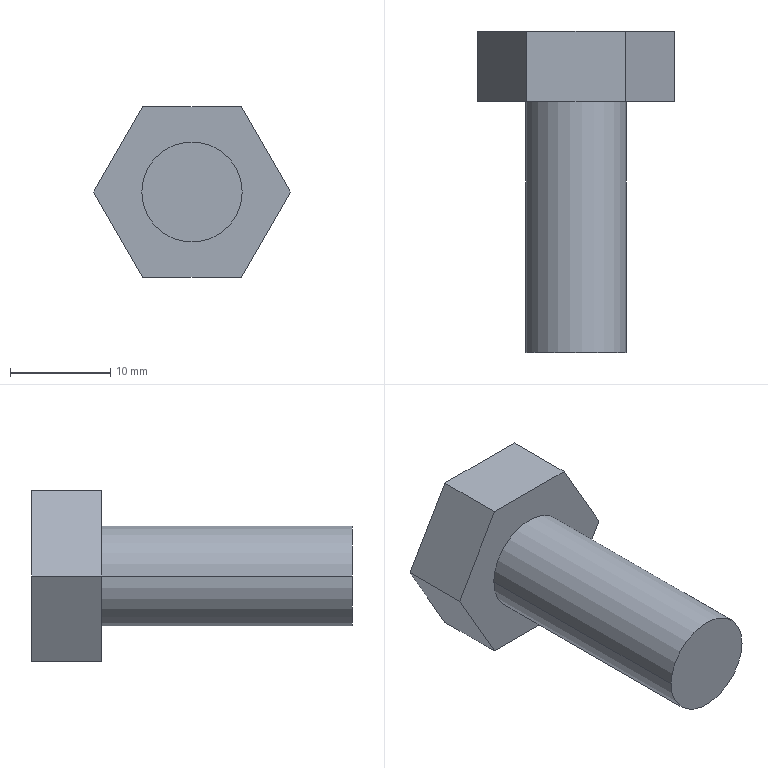Part | STEP file | LIB_27897312_M10X25 | 1 solid | 11 faces | box 19.63 x 32 x 17 mm | volume 3715 mm3 | plane 9 | cylinder 2 | commonest cylinder face diameters 10 x2
STEP:
#1=CARTESIAN_POINT('',(0.,0.,0.));
#2=DIRECTION('',(0.,0.,1.));
#3=DIRECTION('',(1.,0.,0.));
#4=AXIS2_PLACEMENT_3D('',#1,#2,#3);
#5=CARTESIAN_POINT('',(-4.907,0.,-8.5));
#6=VERTEX_POINT('',#5);
#7=CARTESIAN_POINT('',(-9.815,0.,0.));
#8=VERTEX_POINT('',#7);
#9=CARTESIAN_POINT('',(-4.907,0.,-8.5));
#10=DIRECTION('',(-0.5,0.,0.866));
#11=VECTOR('',#10,1.);
#12=LINE('',#9,#11);
#13=CARTESIAN_POINT('',(0.,0.,0.));
#14=DIRECTION('',(0.,1.,0.));
#15=DIRECTION('',(1.,0.,0.));
#16=AXIS2_PLACEMENT_3D('',#13,#14,#15);
#17=PLANE('',#16);
#18=CARTESIAN_POINT('',(-4.907,8.5));
#19=DIRECTION('',(-0.5,-0.866));
#20=VECTOR('',#19,1.);
#21=LINE('',#18,#20);
#22=(GEOMETRIC_REPRESENTATION_CONTEXT(2)PARAMETRIC_REPRESENTATION_CONTEXT()REPRESENTATION_CONTEXT('',''));
#23=DEFINITIONAL_REPRESENTATION('',(#21),#22);
#24=PCURVE('',#17,#23);
#25=CARTESIAN_POINT('',(-4.907,0.,-8.5));
#26=DIRECTION('',(-0.866,0.,-0.5));
#27=DIRECTION('',(-0.5,0.,0.866));
#28=AXIS2_PLACEMENT_3D('',#25,#26,#27);
#29=PLANE('',#28);
#30=CARTESIAN_POINT('',(0.,0.));
#31=DIRECTION('',(1.,0.));
#32=VECTOR('',#31,1.);
#33=LINE('',#30,#32);
#34=(GEOMETRIC_REPRESENTATION_CONTEXT(2)PARAMETRIC_REPRESENTATION_CONTEXT()REPRESENTATION_CONTEXT('',''));
#35=DEFINITIONAL_REPRESENTATION('',(#33),#34);
#36=PCURVE('',#29,#35);
#37=SURFACE_CURVE('',#12,(#24,#36),.PCURVE_S1.);
#38=EDGE_CURVE('',#6,#8,#37,.T.);
#39=ORIENTED_EDGE('',*,*,#38,.T.);
#40=CARTESIAN_POINT('',(-4.907,0.,8.5));
#41=VERTEX_POINT('',#40);
#42=CARTESIAN_POINT('',(-9.815,0.,0.));
#43=DIRECTION('',(0.5,0.,0.866));
#44=VECTOR('',#43,1.);
#45=LINE('',#42,#44);
#46=CARTESIAN_POINT('',(-9.815,0.));
#47=DIRECTION('',(0.5,-0.866));
#48=VECTOR('',#47,1.);
#49=LINE('',#46,#48);
#50=(GEOMETRIC_REPRESENTATION_CONTEXT(2)PARAMETRIC_REPRESENTATION_CONTEXT()REPRESENTATION_CONTEXT('',''));
#51=DEFINITIONAL_REPRESENTATION('',(#49),#50);
#52=PCURVE('',#17,#51);
#53=CARTESIAN_POINT('',(-9.815,0.,0.));
#54=DIRECTION('',(-0.866,0.,0.5));
#55=DIRECTION('',(0.5,0.,0.866));
#56=AXIS2_PLACEMENT_3D('',#53,#54,#55);
#57=PLANE('',#56);
#58=CARTESIAN_POINT('',(0.,0.));
#59=DIRECTION('',(1.,0.));
#60=VECTOR('',#59,1.);
#61=LINE('',#58,#60);
#62=(GEOMETRIC_REPRESENTATION_CONTEXT(2)PARAMETRIC_REPRESENTATION_CONTEXT()REPRESENTATION_CONTEXT('',''));
#63=DEFINITIONAL_REPRESENTATION('',(#61),#62);
#64=PCURVE('',#57,#63);
#65=SURFACE_CURVE('',#45,(#52,#64),.PCURVE_S1.);
#66=EDGE_CURVE('',#8,#41,#65,.T.);
#67=ORIENTED_EDGE('',*,*,#66,.T.);
#68=CARTESIAN_POINT('',(4.907,0.,8.5));
#69=VERTEX_POINT('',#68);
#70=CARTESIAN_POINT('',(-4.907,0.,8.5));
#71=DIRECTION('',(1.,0.,0.));
#72=VECTOR('',#71,1.);
#73=LINE('',#70,#72);
#74=CARTESIAN_POINT('',(-4.907,-8.5));
#75=DIRECTION('',(1.,0.));
#76=VECTOR('',#75,1.);
#77=LINE('',#74,#76);
#78=(GEOMETRIC_REPRESENTATION_CONTEXT(2)PARAMETRIC_REPRESENTATION_CONTEXT()REPRESENTATION_CONTEXT('',''));
#79=DEFINITIONAL_REPRESENTATION('',(#77),#78);
#80=PCURVE('',#17,#79);
#81=CARTESIAN_POINT('',(-4.907,0.,8.5));
#82=DIRECTION('',(0.,0.,1.));
#83=DIRECTION('',(1.,0.,0.));
#84=AXIS2_PLACEMENT_3D('',#81,#82,#83);
#85=PLANE('',#84);
#86=CARTESIAN_POINT('',(0.,0.));
#87=DIRECTION('',(1.,0.));
#88=VECTOR('',#87,1.);
#89=LINE('',#86,#88);
#90=(GEOMETRIC_REPRESENTATION_CONTEXT(2)PARAMETRIC_REPRESENTATION_CONTEXT()REPRESENTATION_CONTEXT('',''));
#91=DEFINITIONAL_REPRESENTATION('',(#89),#90);
#92=PCURVE('',#85,#91);
#93=SURFACE_CURVE('',#73,(#80,#92),.PCURVE_S1.);
#94=EDGE_CURVE('',#41,#69,#93,.T.);
#95=ORIENTED_EDGE('',*,*,#94,.T.);
#96=CARTESIAN_POINT('',(9.815,0.,0.));
#97=VERTEX_POINT('',#96);
#98=CARTESIAN_POINT('',(4.907,0.,8.5));
#99=DIRECTION('',(0.5,0.,-0.866));
#100=VECTOR('',#99,1.);
#101=LINE('',#98,#100);
#102=CARTESIAN_POINT('',(4.907,-8.5));
#103=DIRECTION('',(0.5,0.866));
#104=VECTOR('',#103,1.);
#105=LINE('',#102,#104);
#106=(GEOMETRIC_REPRESENTATION_CONTEXT(2)PARAMETRIC_REPRESENTATION_CONTEXT()REPRESENTATION_CONTEXT('',''));
#107=DEFINITIONAL_REPRESENTATION('',(#105),#106);
#108=PCURVE('',#17,#107);
#109=CARTESIAN_POINT('',(4.907,0.,8.5));
#110=DIRECTION('',(0.866,0.,0.5));
#111=DIRECTION('',(0.5,0.,-0.866));
#112=AXIS2_PLACEMENT_3D('',#109,#110,#111);
#113=PLANE('',#112);
#114=CARTESIAN_POINT('',(0.,0.));
#115=DIRECTION('',(1.,0.));
#116=VECTOR('',#115,1.);
#117=LINE('',#114,#116);
#118=(GEOMETRIC_REPRESENTATION_CONTEXT(2)PARAMETRIC_REPRESENTATION_CONTEXT()REPRESENTATION_CONTEXT('',''));
#119=DEFINITIONAL_REPRESENTATION('',(#117),#118);
#120=PCURVE('',#113,#119);
#121=SURFACE_CURVE('',#101,(#108,#120),.PCURVE_S1.);
#122=EDGE_CURVE('',#69,#97,#121,.T.);
#123=ORIENTED_EDGE('',*,*,#122,.T.);
#124=CARTESIAN_POINT('',(4.907,0.,-8.5));
#125=VERTEX_POINT('',#124);
#126=CARTESIAN_POINT('',(9.815,0.,0.));
#127=DIRECTION('',(-0.5,0.,-0.866));
#128=VECTOR('',#127,1.);
#129=LINE('',#126,#128);
#130=CARTESIAN_POINT('',(9.815,0.));
#131=DIRECTION('',(-0.5,0.866));
#132=VECTOR('',#131,1.);
#133=LINE('',#130,#132);
#134=(GEOMETRIC_REPRESENTATION_CONTEXT(2)PARAMETRIC_REPRESENTATION_CONTEXT()REPRESENTATION_CONTEXT('',''));
#135=DEFINITIONAL_REPRESENTATION('',(#133),#134);
#136=PCURVE('',#17,#135);
#137=CARTESIAN_POINT('',(9.815,0.,0.));
#138=DIRECTION('',(0.866,0.,-0.5));
#139=DIRECTION('',(-0.5,0.,-0.866));
#140=AXIS2_PLACEMENT_3D('',#137,#138,#139);
#141=PLANE('',#140);
#142=CARTESIAN_POINT('',(0.,0.));
#143=DIRECTION('',(1.,0.));
#144=VECTOR('',#143,1.);
#145=LINE('',#142,#144);
#146=(GEOMETRIC_REPRESENTATION_CONTEXT(2)PARAMETRIC_REPRESENTATION_CONTEXT()REPRESENTATION_CONTEXT('',''));
#147=DEFINITIONAL_REPRESENTATION('',(#145),#146);
#148=PCURVE('',#141,#147);
#149=SURFACE_CURVE('',#129,(#136,#148),.PCURVE_S1.);
#150=EDGE_CURVE('',#97,#125,#149,.T.);
#151=ORIENTED_EDGE('',*,*,#150,.T.);
#152=CARTESIAN_POINT('',(4.907,0.,-8.5));
#153=DIRECTION('',(-1.,0.,0.));
#154=VECTOR('',#153,1.);
#155=LINE('',#152,#154);
#156=CARTESIAN_POINT('',(4.907,8.5));
#157=DIRECTION('',(-1.,0.));
#158=VECTOR('',#157,1.);
#159=LINE('',#156,#158);
#160=(GEOMETRIC_REPRESENTATION_CONTEXT(2)PARAMETRIC_REPRESENTATION_CONTEXT()REPRESENTATION_CONTEXT('',''));
#161=DEFINITIONAL_REPRESENTATION('',(#159),#160);
#162=PCURVE('',#17,#161);
#163=CARTESIAN_POINT('',(4.907,0.,-8.5));
#164=DIRECTION('',(0.,0.,-1.));
#165=DIRECTION('',(-1.,0.,0.));
#166=AXIS2_PLACEMENT_3D('',#163,#164,#165);
#167=PLANE('',#166);
#168=CARTESIAN_POINT('',(0.,0.));
#169=DIRECTION('',(1.,0.));
#170=VECTOR('',#169,1.);
#171=LINE('',#168,#170);
#172=(GEOMETRIC_REPRESENTATION_CONTEXT(2)PARAMETRIC_REPRESENTATION_CONTEXT()REPRESENTATION_CONTEXT('',''));
#173=DEFINITIONAL_REPRESENTATION('',(#171),#172);
#174=PCURVE('',#167,#173);
#175=SURFACE_CURVE('',#155,(#162,#174),.PCURVE_S1.);
#176=EDGE_CURVE('',#125,#6,#175,.T.);
#177=ORIENTED_EDGE('',*,*,#176,.T.);
#178=EDGE_LOOP('',(#39,#67,#95,#123,#151,#177));
#179=FACE_BOUND('',#178,.F.);
#180=CARTESIAN_POINT('',(5.,0.,0.));
#181=VERTEX_POINT('',#180);
#182=CARTESIAN_POINT('',(-5.,0.,0.));
#183=VERTEX_POINT('',#182);
#184=CARTESIAN_POINT('',(0.,0.,0.));
#185=DIRECTION('',(0.,-1.,0.));
#186=DIRECTION('',(1.,0.,0.));
#187=AXIS2_PLACEMENT_3D('',#184,#185,#186);
#188=CIRCLE('',#187,5.);
#189=CARTESIAN_POINT('',(5.,0.));
#190=CARTESIAN_POINT('',(5.,-8.66));
#191=CARTESIAN_POINT('',(-2.5,-4.33));
#192=CARTESIAN_POINT('',(-10.,0.));
#193=CARTESIAN_POINT('',(-2.5,4.33));
#194=CARTESIAN_POINT('',(5.,8.66));
#195=CARTESIAN_POINT('',(5.,0.));
#196=(BOUNDED_CURVE()B_SPLINE_CURVE(2,(#189,#190,#191,#192,#193,#194,#195),.UNSPECIFIED.,.T.,.F.)B_SPLINE_CURVE_WITH_KNOTS((1,2,2,2,2,1),(-2.094,0.,2.094,4.189,6.283,8.378),.UNSPECIFIED.)CURVE()GEOMETRIC_REPRESENTATION_ITEM()RATIONAL_B_SPLINE_CURVE((1.,0.5,1.,0.5,1.,0.5,1.))REPRESENTATION_ITEM(''));
#197=(GEOMETRIC_REPRESENTATION_CONTEXT(2)PARAMETRIC_REPRESENTATION_CONTEXT()REPRESENTATION_CONTEXT('',''));
#198=DEFINITIONAL_REPRESENTATION('',(#196),#197);
#199=PCURVE('',#17,#198);
#200=CARTESIAN_POINT('',(0.,0.,0.));
#201=DIRECTION('',(0.,-1.,0.));
#202=DIRECTION('',(1.,0.,0.));
#203=AXIS2_PLACEMENT_3D('',#200,#201,#202);
#204=CYLINDRICAL_SURFACE('',#203,5.);
#205=CARTESIAN_POINT('',(0.,0.));
#206=DIRECTION('',(1.,0.));
#207=VECTOR('',#206,1.);
#208=LINE('',#205,#207);
#209=(GEOMETRIC_REPRESENTATION_CONTEXT(2)PARAMETRIC_REPRESENTATION_CONTEXT()REPRESENTATION_CONTEXT('',''));
#210=DEFINITIONAL_REPRESENTATION('',(#208),#209);
#211=PCURVE('',#204,#210);
#212=SURFACE_CURVE('',#188,(#199,#211),.PCURVE_S1.);
#213=EDGE_CURVE('',#181,#183,#212,.T.);
#214=ORIENTED_EDGE('',*,*,#213,.T.);
#215=CARTESIAN_POINT('',(0.,0.,0.));
#216=DIRECTION('',(0.,-1.,0.));
#217=DIRECTION('',(-1.,0.,0.));
#218=AXIS2_PLACEMENT_3D('',#215,#216,#217);
#219=CIRCLE('',#218,5.);
#220=CARTESIAN_POINT('',(-5.,0.));
#221=CARTESIAN_POINT('',(-5.,8.66));
#222=CARTESIAN_POINT('',(2.5,4.33));
#223=CARTESIAN_POINT('',(10.,0.));
#224=CARTESIAN_POINT('',(2.5,-4.33));
#225=CARTESIAN_POINT('',(-5.,-8.66));
#226=CARTESIAN_POINT('',(-5.,0.));
#227=(BOUNDED_CURVE()B_SPLINE_CURVE(2,(#220,#221,#222,#223,#224,#225,#226),.UNSPECIFIED.,.T.,.F.)B_SPLINE_CURVE_WITH_KNOTS((1,2,2,2,2,1),(-2.094,0.,2.094,4.189,6.283,8.378),.UNSPECIFIED.)CURVE()GEOMETRIC_REPRESENTATION_ITEM()RATIONAL_B_SPLINE_CURVE((1.,0.5,1.,0.5,1.,0.5,1.))REPRESENTATION_ITEM(''));
#228=(GEOMETRIC_REPRESENTATION_CONTEXT(2)PARAMETRIC_REPRESENTATION_CONTEXT()REPRESENTATION_CONTEXT('',''));
#229=DEFINITIONAL_REPRESENTATION('',(#227),#228);
#230=PCURVE('',#17,#229);
#231=CARTESIAN_POINT('',(0.,0.,0.));
#232=DIRECTION('',(0.,-1.,0.));
#233=DIRECTION('',(1.,0.,0.));
#234=AXIS2_PLACEMENT_3D('',#231,#232,#233);
#235=CYLINDRICAL_SURFACE('',#234,5.);
#236=CARTESIAN_POINT('',(3.142,0.));
#237=DIRECTION('',(1.,0.));
#238=VECTOR('',#237,1.);
#239=LINE('',#236,#238);
#240=(GEOMETRIC_REPRESENTATION_CONTEXT(2)PARAMETRIC_REPRESENTATION_CONTEXT()REPRESENTATION_CONTEXT('',''));
#241=DEFINITIONAL_REPRESENTATION('',(#239),#240);
#242=PCURVE('',#235,#241);
#243=SURFACE_CURVE('',#219,(#230,#242),.PCURVE_S1.);
#244=EDGE_CURVE('',#183,#181,#243,.T.);
#245=ORIENTED_EDGE('',*,*,#244,.T.);
#246=EDGE_LOOP('',(#214,#245));
#247=FACE_BOUND('',#246,.F.);
#248=ADVANCED_FACE('',(#179,#247),#17,.F.);
#249=ORIENTED_EDGE('',*,*,#38,.F.);
#250=CARTESIAN_POINT('',(-4.907,7.,-8.5));
#251=VERTEX_POINT('',#250);
#252=CARTESIAN_POINT('',(-4.907,0.,-8.5));
#253=DIRECTION('',(0.,1.,0.));
#254=VECTOR('',#253,1.);
#255=LINE('',#252,#254);
#256=CARTESIAN_POINT('',(0.,0.));
#257=DIRECTION('',(0.,1.));
#258=VECTOR('',#257,1.);
#259=LINE('',#256,#258);
#260=(GEOMETRIC_REPRESENTATION_CONTEXT(2)PARAMETRIC_REPRESENTATION_CONTEXT()REPRESENTATION_CONTEXT('',''));
#261=DEFINITIONAL_REPRESENTATION('',(#259),#260);
#262=PCURVE('',#29,#261);
#263=CARTESIAN_POINT('',(9.815,0.));
#264=DIRECTION('',(0.,1.));
#265=VECTOR('',#264,1.);
#266=LINE('',#263,#265);
#267=(GEOMETRIC_REPRESENTATION_CONTEXT(2)PARAMETRIC_REPRESENTATION_CONTEXT()REPRESENTATION_CONTEXT('',''));
#268=DEFINITIONAL_REPRESENTATION('',(#266),#267);
#269=PCURVE('',#167,#268);
#270=SURFACE_CURVE('',#255,(#262,#269),.PCURVE_S1.);
#271=EDGE_CURVE('',#6,#251,#270,.T.);
#272=ORIENTED_EDGE('',*,*,#271,.T.);
#273=CARTESIAN_POINT('',(-9.815,7.,0.));
#274=VERTEX_POINT('',#273);
#275=CARTESIAN_POINT('',(-4.907,7.,-8.5));
#276=DIRECTION('',(-0.5,0.,0.866));
#277=VECTOR('',#276,1.);
#278=LINE('',#275,#277);
#279=CARTESIAN_POINT('',(0.,7.));
#280=DIRECTION('',(1.,0.));
#281=VECTOR('',#280,1.);
#282=LINE('',#279,#281);
#283=(GEOMETRIC_REPRESENTATION_CONTEXT(2)PARAMETRIC_REPRESENTATION_CONTEXT()REPRESENTATION_CONTEXT('',''));
#284=DEFINITIONAL_REPRESENTATION('',(#282),#283);
#285=PCURVE('',#29,#284);
#286=CARTESIAN_POINT('',(0.,7.,0.));
#287=DIRECTION('',(0.,1.,0.));
#288=DIRECTION('',(1.,0.,0.));
#289=AXIS2_PLACEMENT_3D('',#286,#287,#288);
#290=PLANE('',#289);
#291=CARTESIAN_POINT('',(-4.907,8.5));
#292=DIRECTION('',(-0.5,-0.866));
#293=VECTOR('',#292,1.);
#294=LINE('',#291,#293);
#295=(GEOMETRIC_REPRESENTATION_CONTEXT(2)PARAMETRIC_REPRESENTATION_CONTEXT()REPRESENTATION_CONTEXT('',''));
#296=DEFINITIONAL_REPRESENTATION('',(#294),#295);
#297=PCURVE('',#290,#296);
#298=SURFACE_CURVE('',#278,(#285,#297),.PCURVE_S1.);
#299=EDGE_CURVE('',#251,#274,#298,.T.);
#300=ORIENTED_EDGE('',*,*,#299,.T.);
#301=CARTESIAN_POINT('',(-9.815,0.,0.));
#302=DIRECTION('',(0.,1.,0.));
#303=VECTOR('',#302,1.);
#304=LINE('',#301,#303);
#305=CARTESIAN_POINT('',(9.815,0.));
#306=DIRECTION('',(0.,1.));
#307=VECTOR('',#306,1.);
#308=LINE('',#305,#307);
#309=(GEOMETRIC_REPRESENTATION_CONTEXT(2)PARAMETRIC_REPRESENTATION_CONTEXT()REPRESENTATION_CONTEXT('',''));
#310=DEFINITIONAL_REPRESENTATION('',(#308),#309);
#311=PCURVE('',#29,#310);
#312=CARTESIAN_POINT('',(0.,0.));
#313=DIRECTION('',(0.,1.));
#314=VECTOR('',#313,1.);
#315=LINE('',#312,#314);
#316=(GEOMETRIC_REPRESENTATION_CONTEXT(2)PARAMETRIC_REPRESENTATION_CONTEXT()REPRESENTATION_CONTEXT('',''));
#317=DEFINITIONAL_REPRESENTATION('',(#315),#316);
#318=PCURVE('',#57,#317);
#319=SURFACE_CURVE('',#304,(#311,#318),.PCURVE_S1.);
#320=EDGE_CURVE('',#8,#274,#319,.T.);
#321=ORIENTED_EDGE('',*,*,#320,.F.);
#322=EDGE_LOOP('',(#249,#272,#300,#321));
#323=FACE_BOUND('',#322,.F.);
#324=ADVANCED_FACE('',(#323),#29,.T.);
#325=ORIENTED_EDGE('',*,*,#176,.F.);
#326=CARTESIAN_POINT('',(4.907,7.,-8.5));
#327=VERTEX_POINT('',#326);
#328=CARTESIAN_POINT('',(4.907,0.,-8.5));
#329=DIRECTION('',(0.,1.,0.));
#330=VECTOR('',#329,1.);
#331=LINE('',#328,#330);
#332=CARTESIAN_POINT('',(0.,0.));
#333=DIRECTION('',(0.,1.));
#334=VECTOR('',#333,1.);
#335=LINE('',#332,#334);
#336=(GEOMETRIC_REPRESENTATION_CONTEXT(2)PARAMETRIC_REPRESENTATION_CONTEXT()REPRESENTATION_CONTEXT('',''));
#337=DEFINITIONAL_REPRESENTATION('',(#335),#336);
#338=PCURVE('',#167,#337);
#339=CARTESIAN_POINT('',(9.815,0.));
#340=DIRECTION('',(0.,1.));
#341=VECTOR('',#340,1.);
#342=LINE('',#339,#341);
#343=(GEOMETRIC_REPRESENTATION_CONTEXT(2)PARAMETRIC_REPRESENTATION_CONTEXT()REPRESENTATION_CONTEXT('',''));
#344=DEFINITIONAL_REPRESENTATION('',(#342),#343);
#345=PCURVE('',#141,#344);
#346=SURFACE_CURVE('',#331,(#338,#345),.PCURVE_S1.);
#347=EDGE_CURVE('',#125,#327,#346,.T.);
#348=ORIENTED_EDGE('',*,*,#347,.T.);
#349=CARTESIAN_POINT('',(4.907,7.,-8.5));
#350=DIRECTION('',(-1.,0.,0.));
#351=VECTOR('',#350,1.);
#352=LINE('',#349,#351);
#353=CARTESIAN_POINT('',(0.,7.));
#354=DIRECTION('',(1.,0.));
#355=VECTOR('',#354,1.);
#356=LINE('',#353,#355);
#357=(GEOMETRIC_REPRESENTATION_CONTEXT(2)PARAMETRIC_REPRESENTATION_CONTEXT()REPRESENTATION_CONTEXT('',''));
#358=DEFINITIONAL_REPRESENTATION('',(#356),#357);
#359=PCURVE('',#167,#358);
#360=CARTESIAN_POINT('',(4.907,8.5));
#361=DIRECTION('',(-1.,0.));
#362=VECTOR('',#361,1.);
#363=LINE('',#360,#362);
#364=(GEOMETRIC_REPRESENTATION_CONTEXT(2)PARAMETRIC_REPRESENTATION_CONTEXT()REPRESENTATION_CONTEXT('',''));
#365=DEFINITIONAL_REPRESENTATION('',(#363),#364);
#366=PCURVE('',#290,#365);
#367=SURFACE_CURVE('',#352,(#359,#366),.PCURVE_S1.);
#368=EDGE_CURVE('',#327,#251,#367,.T.);
#369=ORIENTED_EDGE('',*,*,#368,.T.);
#370=ORIENTED_EDGE('',*,*,#271,.F.);
#371=EDGE_LOOP('',(#325,#348,#369,#370));
#372=FACE_BOUND('',#371,.F.);
#373=ADVANCED_FACE('',(#372),#167,.T.);
#374=ORIENTED_EDGE('',*,*,#150,.F.);
#375=CARTESIAN_POINT('',(9.815,7.,0.));
#376=VERTEX_POINT('',#375);
#377=CARTESIAN_POINT('',(9.815,0.,0.));
#378=DIRECTION('',(0.,1.,0.));
#379=VECTOR('',#378,1.);
#380=LINE('',#377,#379);
#381=CARTESIAN_POINT('',(0.,0.));
#382=DIRECTION('',(0.,1.));
#383=VECTOR('',#382,1.);
#384=LINE('',#381,#383);
#385=(GEOMETRIC_REPRESENTATION_CONTEXT(2)PARAMETRIC_REPRESENTATION_CONTEXT()REPRESENTATION_CONTEXT('',''));
#386=DEFINITIONAL_REPRESENTATION('',(#384),#385);
#387=PCURVE('',#141,#386);
#388=CARTESIAN_POINT('',(9.815,0.));
#389=DIRECTION('',(0.,1.));
#390=VECTOR('',#389,1.);
#391=LINE('',#388,#390);
#392=(GEOMETRIC_REPRESENTATION_CONTEXT(2)PARAMETRIC_REPRESENTATION_CONTEXT()REPRESENTATION_CONTEXT('',''));
#393=DEFINITIONAL_REPRESENTATION('',(#391),#392);
#394=PCURVE('',#113,#393);
#395=SURFACE_CURVE('',#380,(#387,#394),.PCURVE_S1.);
#396=EDGE_CURVE('',#97,#376,#395,.T.);
#397=ORIENTED_EDGE('',*,*,#396,.T.);
#398=CARTESIAN_POINT('',(9.815,7.,0.));
#399=DIRECTION('',(-0.5,0.,-0.866));
#400=VECTOR('',#399,1.);
#401=LINE('',#398,#400);
#402=CARTESIAN_POINT('',(0.,7.));
#403=DIRECTION('',(1.,0.));
#404=VECTOR('',#403,1.);
#405=LINE('',#402,#404);
#406=(GEOMETRIC_REPRESENTATION_CONTEXT(2)PARAMETRIC_REPRESENTATION_CONTEXT()REPRESENTATION_CONTEXT('',''));
#407=DEFINITIONAL_REPRESENTATION('',(#405),#406);
#408=PCURVE('',#141,#407);
#409=CARTESIAN_POINT('',(9.815,0.));
#410=DIRECTION('',(-0.5,0.866));
#411=VECTOR('',#410,1.);
#412=LINE('',#409,#411);
#413=(GEOMETRIC_REPRESENTATION_CONTEXT(2)PARAMETRIC_REPRESENTATION_CONTEXT()REPRESENTATION_CONTEXT('',''));
#414=DEFINITIONAL_REPRESENTATION('',(#412),#413);
#415=PCURVE('',#290,#414);
#416=SURFACE_CURVE('',#401,(#408,#415),.PCURVE_S1.);
#417=EDGE_CURVE('',#376,#327,#416,.T.);
#418=ORIENTED_EDGE('',*,*,#417,.T.);
#419=ORIENTED_EDGE('',*,*,#347,.F.);
#420=EDGE_LOOP('',(#374,#397,#418,#419));
#421=FACE_BOUND('',#420,.F.);
#422=ADVANCED_FACE('',(#421),#141,.T.);
#423=ORIENTED_EDGE('',*,*,#122,.F.);
#424=CARTESIAN_POINT('',(4.907,7.,8.5));
#425=VERTEX_POINT('',#424);
#426=CARTESIAN_POINT('',(4.907,0.,8.5));
#427=DIRECTION('',(0.,1.,0.));
#428=VECTOR('',#427,1.);
#429=LINE('',#426,#428);
#430=CARTESIAN_POINT('',(0.,0.));
#431=DIRECTION('',(0.,1.));
#432=VECTOR('',#431,1.);
#433=LINE('',#430,#432);
#434=(GEOMETRIC_REPRESENTATION_CONTEXT(2)PARAMETRIC_REPRESENTATION_CONTEXT()REPRESENTATION_CONTEXT('',''));
#435=DEFINITIONAL_REPRESENTATION('',(#433),#434);
#436=PCURVE('',#113,#435);
#437=CARTESIAN_POINT('',(9.815,0.));
#438=DIRECTION('',(0.,1.));
#439=VECTOR('',#438,1.);
#440=LINE('',#437,#439);
#441=(GEOMETRIC_REPRESENTATION_CONTEXT(2)PARAMETRIC_REPRESENTATION_CONTEXT()REPRESENTATION_CONTEXT('',''));
#442=DEFINITIONAL_REPRESENTATION('',(#440),#441);
#443=PCURVE('',#85,#442);
#444=SURFACE_CURVE('',#429,(#436,#443),.PCURVE_S1.);
#445=EDGE_CURVE('',#69,#425,#444,.T.);
#446=ORIENTED_EDGE('',*,*,#445,.T.);
#447=CARTESIAN_POINT('',(4.907,7.,8.5));
#448=DIRECTION('',(0.5,0.,-0.866));
#449=VECTOR('',#448,1.);
#450=LINE('',#447,#449);
#451=CARTESIAN_POINT('',(0.,7.));
#452=DIRECTION('',(1.,0.));
#453=VECTOR('',#452,1.);
#454=LINE('',#451,#453);
#455=(GEOMETRIC_REPRESENTATION_CONTEXT(2)PARAMETRIC_REPRESENTATION_CONTEXT()REPRESENTATION_CONTEXT('',''));
#456=DEFINITIONAL_REPRESENTATION('',(#454),#455);
#457=PCURVE('',#113,#456);
#458=CARTESIAN_POINT('',(4.907,-8.5));
#459=DIRECTION('',(0.5,0.866));
#460=VECTOR('',#459,1.);
#461=LINE('',#458,#460);
#462=(GEOMETRIC_REPRESENTATION_CONTEXT(2)PARAMETRIC_REPRESENTATION_CONTEXT()REPRESENTATION_CONTEXT('',''));
#463=DEFINITIONAL_REPRESENTATION('',(#461),#462);
#464=PCURVE('',#290,#463);
#465=SURFACE_CURVE('',#450,(#457,#464),.PCURVE_S1.);
#466=EDGE_CURVE('',#425,#376,#465,.T.);
#467=ORIENTED_EDGE('',*,*,#466,.T.);
#468=ORIENTED_EDGE('',*,*,#396,.F.);
#469=EDGE_LOOP('',(#423,#446,#467,#468));
#470=FACE_BOUND('',#469,.F.);
#471=ADVANCED_FACE('',(#470),#113,.T.);
#472=ORIENTED_EDGE('',*,*,#94,.F.);
#473=CARTESIAN_POINT('',(-4.907,7.,8.5));
#474=VERTEX_POINT('',#473);
#475=CARTESIAN_POINT('',(-4.907,0.,8.5));
#476=DIRECTION('',(0.,1.,0.));
#477=VECTOR('',#476,1.);
#478=LINE('',#475,#477);
#479=CARTESIAN_POINT('',(0.,0.));
#480=DIRECTION('',(0.,1.));
#481=VECTOR('',#480,1.);
#482=LINE('',#479,#481);
#483=(GEOMETRIC_REPRESENTATION_CONTEXT(2)PARAMETRIC_REPRESENTATION_CONTEXT()REPRESENTATION_CONTEXT('',''));
#484=DEFINITIONAL_REPRESENTATION('',(#482),#483);
#485=PCURVE('',#85,#484);
#486=CARTESIAN_POINT('',(9.815,0.));
#487=DIRECTION('',(0.,1.));
#488=VECTOR('',#487,1.);
#489=LINE('',#486,#488);
#490=(GEOMETRIC_REPRESENTATION_CONTEXT(2)PARAMETRIC_REPRESENTATION_CONTEXT()REPRESENTATION_CONTEXT('',''));
#491=DEFINITIONAL_REPRESENTATION('',(#489),#490);
#492=PCURVE('',#57,#491);
#493=SURFACE_CURVE('',#478,(#485,#492),.PCURVE_S1.);
#494=EDGE_CURVE('',#41,#474,#493,.T.);
#495=ORIENTED_EDGE('',*,*,#494,.T.);
#496=CARTESIAN_POINT('',(-4.907,7.,8.5));
#497=DIRECTION('',(1.,0.,0.));
#498=VECTOR('',#497,1.);
#499=LINE('',#496,#498);
#500=CARTESIAN_POINT('',(0.,7.));
#501=DIRECTION('',(1.,0.));
#502=VECTOR('',#501,1.);
#503=LINE('',#500,#502);
#504=(GEOMETRIC_REPRESENTATION_CONTEXT(2)PARAMETRIC_REPRESENTATION_CONTEXT()REPRESENTATION_CONTEXT('',''));
#505=DEFINITIONAL_REPRESENTATION('',(#503),#504);
#506=PCURVE('',#85,#505);
#507=CARTESIAN_POINT('',(-4.907,-8.5));
#508=DIRECTION('',(1.,0.));
#509=VECTOR('',#508,1.);
#510=LINE('',#507,#509);
#511=(GEOMETRIC_REPRESENTATION_CONTEXT(2)PARAMETRIC_REPRESENTATION_CONTEXT()REPRESENTATION_CONTEXT('',''));
#512=DEFINITIONAL_REPRESENTATION('',(#510),#511);
#513=PCURVE('',#290,#512);
#514=SURFACE_CURVE('',#499,(#506,#513),.PCURVE_S1.);
#515=EDGE_CURVE('',#474,#425,#514,.T.);
#516=ORIENTED_EDGE('',*,*,#515,.T.);
#517=ORIENTED_EDGE('',*,*,#445,.F.);
#518=EDGE_LOOP('',(#472,#495,#516,#517));
#519=FACE_BOUND('',#518,.F.);
#520=ADVANCED_FACE('',(#519),#85,.T.);
#521=ORIENTED_EDGE('',*,*,#66,.F.);
#522=ORIENTED_EDGE('',*,*,#320,.T.);
#523=CARTESIAN_POINT('',(-9.815,7.,0.));
#524=DIRECTION('',(0.5,0.,0.866));
#525=VECTOR('',#524,1.);
#526=LINE('',#523,#525);
#527=CARTESIAN_POINT('',(0.,7.));
#528=DIRECTION('',(1.,0.));
#529=VECTOR('',#528,1.);
#530=LINE('',#527,#529);
#531=(GEOMETRIC_REPRESENTATION_CONTEXT(2)PARAMETRIC_REPRESENTATION_CONTEXT()REPRESENTATION_CONTEXT('',''));
#532=DEFINITIONAL_REPRESENTATION('',(#530),#531);
#533=PCURVE('',#57,#532);
#534=CARTESIAN_POINT('',(-9.815,0.));
#535=DIRECTION('',(0.5,-0.866));
#536=VECTOR('',#535,1.);
#537=LINE('',#534,#536);
#538=(GEOMETRIC_REPRESENTATION_CONTEXT(2)PARAMETRIC_REPRESENTATION_CONTEXT()REPRESENTATION_CONTEXT('',''));
#539=DEFINITIONAL_REPRESENTATION('',(#537),#538);
#540=PCURVE('',#290,#539);
#541=SURFACE_CURVE('',#526,(#533,#540),.PCURVE_S1.);
#542=EDGE_CURVE('',#274,#474,#541,.T.);
#543=ORIENTED_EDGE('',*,*,#542,.T.);
#544=ORIENTED_EDGE('',*,*,#494,.F.);
#545=EDGE_LOOP('',(#521,#522,#543,#544));
#546=FACE_BOUND('',#545,.F.);
#547=ADVANCED_FACE('',(#546),#57,.T.);
#548=ORIENTED_EDGE('',*,*,#299,.F.);
#549=ORIENTED_EDGE('',*,*,#368,.F.);
#550=ORIENTED_EDGE('',*,*,#417,.F.);
#551=ORIENTED_EDGE('',*,*,#466,.F.);
#552=ORIENTED_EDGE('',*,*,#515,.F.);
#553=ORIENTED_EDGE('',*,*,#542,.F.);
#554=EDGE_LOOP('',(#548,#549,#550,#551,#552,#553));
#555=FACE_BOUND('',#554,.F.);
#556=ADVANCED_FACE('',(#555),#290,.T.);
#557=CARTESIAN_POINT('',(-5.,-25.,0.));
#558=VERTEX_POINT('',#557);
#559=CARTESIAN_POINT('',(-5.,0.,0.));
#560=DIRECTION('',(0.,-1.,0.));
#561=VECTOR('',#560,1.);
#562=LINE('',#559,#561);
#563=CARTESIAN_POINT('',(3.142,0.));
#564=DIRECTION('',(0.,1.));
#565=VECTOR('',#564,1.);
#566=LINE('',#563,#565);
#567=(GEOMETRIC_REPRESENTATION_CONTEXT(2)PARAMETRIC_REPRESENTATION_CONTEXT()REPRESENTATION_CONTEXT('',''));
#568=DEFINITIONAL_REPRESENTATION('',(#566),#567);
#569=PCURVE('',#204,#568);
#570=CARTESIAN_POINT('',(3.142,0.));
#571=DIRECTION('',(0.,1.));
#572=VECTOR('',#571,1.);
#573=LINE('',#570,#572);
#574=(GEOMETRIC_REPRESENTATION_CONTEXT(2)PARAMETRIC_REPRESENTATION_CONTEXT()REPRESENTATION_CONTEXT('',''));
#575=DEFINITIONAL_REPRESENTATION('',(#573),#574);
#576=PCURVE('',#235,#575);
#577=SURFACE_CURVE('',#562,(#569,#576),.PCURVE_S1.);
#578=EDGE_CURVE('',#183,#558,#577,.T.);
#579=ORIENTED_EDGE('',*,*,#578,.T.);
#580=CARTESIAN_POINT('',(5.,-25.,0.));
#581=VERTEX_POINT('',#580);
#582=CARTESIAN_POINT('',(0.,-25.,0.));
#583=DIRECTION('',(0.,-1.,0.));
#584=DIRECTION('',(1.,0.,0.));
#585=AXIS2_PLACEMENT_3D('',#582,#583,#584);
#586=CIRCLE('',#585,5.);
#587=CARTESIAN_POINT('',(0.,25.));
#588=DIRECTION('',(1.,0.));
#589=VECTOR('',#588,1.);
#590=LINE('',#587,#589);
#591=(GEOMETRIC_REPRESENTATION_CONTEXT(2)PARAMETRIC_REPRESENTATION_CONTEXT()REPRESENTATION_CONTEXT('',''));
#592=DEFINITIONAL_REPRESENTATION('',(#590),#591);
#593=PCURVE('',#204,#592);
#594=CARTESIAN_POINT('',(0.,-25.,0.));
#595=DIRECTION('',(0.,-1.,0.));
#596=DIRECTION('',(1.,0.,0.));
#597=AXIS2_PLACEMENT_3D('',#594,#595,#596);
#598=PLANE('',#597);
#599=CARTESIAN_POINT('',(0.,0.));
#600=DIRECTION('',(1.,0.));
#601=AXIS2_PLACEMENT_2D('',#599,#600);
#602=CIRCLE('',#601,5.);
#603=(GEOMETRIC_REPRESENTATION_CONTEXT(2)PARAMETRIC_REPRESENTATION_CONTEXT()REPRESENTATION_CONTEXT('',''));
#604=DEFINITIONAL_REPRESENTATION('',(#602),#603);
#605=PCURVE('',#598,#604);
#606=SURFACE_CURVE('',#586,(#593,#605),.PCURVE_S1.);
#607=EDGE_CURVE('',#581,#558,#606,.T.);
#608=ORIENTED_EDGE('',*,*,#607,.F.);
#609=CARTESIAN_POINT('',(5.,0.,0.));
#610=DIRECTION('',(0.,-1.,0.));
#611=VECTOR('',#610,1.);
#612=LINE('',#609,#611);
#613=CARTESIAN_POINT('',(0.,0.));
#614=DIRECTION('',(0.,1.));
#615=VECTOR('',#614,1.);
#616=LINE('',#613,#615);
#617=(GEOMETRIC_REPRESENTATION_CONTEXT(2)PARAMETRIC_REPRESENTATION_CONTEXT()REPRESENTATION_CONTEXT('',''));
#618=DEFINITIONAL_REPRESENTATION('',(#616),#617);
#619=PCURVE('',#204,#618);
#620=CARTESIAN_POINT('',(6.283,0.));
#621=DIRECTION('',(0.,1.));
#622=VECTOR('',#621,1.);
#623=LINE('',#620,#622);
#624=(GEOMETRIC_REPRESENTATION_CONTEXT(2)PARAMETRIC_REPRESENTATION_CONTEXT()REPRESENTATION_CONTEXT('',''));
#625=DEFINITIONAL_REPRESENTATION('',(#623),#624);
#626=PCURVE('',#235,#625);
#627=SURFACE_CURVE('',#612,(#619,#626),.PCURVE_S1.);
#628=EDGE_CURVE('',#181,#581,#627,.T.);
#629=ORIENTED_EDGE('',*,*,#628,.F.);
#630=ORIENTED_EDGE('',*,*,#213,.T.);
#631=EDGE_LOOP('',(#579,#608,#629,#630));
#632=FACE_BOUND('',#631,.T.);
#633=ADVANCED_FACE('',(#632),#204,.T.);
#634=ORIENTED_EDGE('',*,*,#628,.T.);
#635=CARTESIAN_POINT('',(0.,-25.,0.));
#636=DIRECTION('',(0.,-1.,0.));
#637=DIRECTION('',(-1.,0.,0.));
#638=AXIS2_PLACEMENT_3D('',#635,#636,#637);
#639=CIRCLE('',#638,5.);
#640=CARTESIAN_POINT('',(3.142,25.));
#641=DIRECTION('',(1.,0.));
#642=VECTOR('',#641,1.);
#643=LINE('',#640,#642);
#644=(GEOMETRIC_REPRESENTATION_CONTEXT(2)PARAMETRIC_REPRESENTATION_CONTEXT()REPRESENTATION_CONTEXT('',''));
#645=DEFINITIONAL_REPRESENTATION('',(#643),#644);
#646=PCURVE('',#235,#645);
#647=CARTESIAN_POINT('',(0.,0.));
#648=DIRECTION('',(-1.,0.));
#649=AXIS2_PLACEMENT_2D('',#647,#648);
#650=CIRCLE('',#649,5.);
#651=(GEOMETRIC_REPRESENTATION_CONTEXT(2)PARAMETRIC_REPRESENTATION_CONTEXT()REPRESENTATION_CONTEXT('',''));
#652=DEFINITIONAL_REPRESENTATION('',(#650),#651);
#653=PCURVE('',#598,#652);
#654=SURFACE_CURVE('',#639,(#646,#653),.PCURVE_S1.);
#655=EDGE_CURVE('',#558,#581,#654,.T.);
#656=ORIENTED_EDGE('',*,*,#655,.F.);
#657=ORIENTED_EDGE('',*,*,#578,.F.);
#658=ORIENTED_EDGE('',*,*,#244,.T.);
#659=EDGE_LOOP('',(#634,#656,#657,#658));
#660=FACE_BOUND('',#659,.T.);
#661=ADVANCED_FACE('',(#660),#235,.T.);
#662=ORIENTED_EDGE('',*,*,#607,.F.);
#663=ORIENTED_EDGE('',*,*,#655,.F.);
#664=EDGE_LOOP('',(#662,#663));
#665=FACE_BOUND('',#664,.F.);
#666=ADVANCED_FACE('',(#665),#598,.T.);
#667=CLOSED_SHELL('',(#248,#324,#373,#422,#471,#520,#547,#556,#633,#661,#666));
#668=MANIFOLD_SOLID_BREP('',#667);
#669=(LENGTH_UNIT()NAMED_UNIT(*)SI_UNIT(.MILLI.,.METRE.));
#670=UNCERTAINTY_MEASURE_WITH_UNIT(LENGTH_MEASURE(0.0000001),#669,'','');
#671=(NAMED_UNIT(*)PLANE_ANGLE_UNIT()SI_UNIT($,.RADIAN.));
#672=(NAMED_UNIT(*)SI_UNIT($,.STERADIAN.)SOLID_ANGLE_UNIT());
#673=(GEOMETRIC_REPRESENTATION_CONTEXT(3)GLOBAL_UNCERTAINTY_ASSIGNED_CONTEXT((#670))GLOBAL_UNIT_ASSIGNED_CONTEXT((#669,#671,#672))REPRESENTATION_CONTEXT('',''));
#674=ADVANCED_BREP_SHAPE_REPRESENTATION('',(#4,#668),#673);